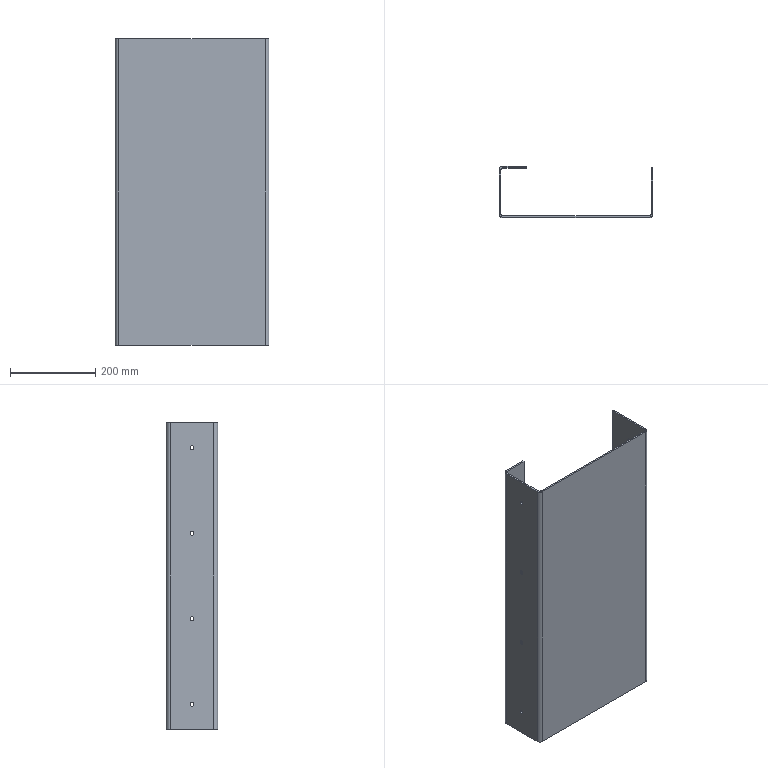Part | SolidWorks | features Extrusion 1, ICE 1 | 1 solid | 34 faces | box 360 x 120 x 716 mm | volume 1828022 mm3 | cylinder 22 | plane 12 | commonest cylinder face diameters 9 x16 10 x3 18 x3
STEP:
#1=CARTESIAN_POINT('',(296.,-55.5,58.));
#2=VERTEX_POINT('',#1);
#3=CARTESIAN_POINT('',(296.,-64.5,58.));
#4=VERTEX_POINT('',#3);
#5=CARTESIAN_POINT('',(296.,-60.,58.));
#6=DIRECTION('',(-1.,0.,0.));
#7=DIRECTION('',(0.,0.,1.));
#8=AXIS2_PLACEMENT_3D('',#5,#6,#7);
#9=CIRCLE('',#8,4.5);
#10=EDGE_CURVE('',#2,#4,#9,.T.);
#11=ORIENTED_EDGE('',*,*,#10,.F.);
#12=CARTESIAN_POINT('',(292.,-55.5,58.));
#13=VERTEX_POINT('',#12);
#14=CARTESIAN_POINT('',(652.,-55.5,58.));
#15=DIRECTION('',(-1.,0.,0.));
#16=VECTOR('',#15,1000.);
#17=LINE('',#14,#16);
#18=EDGE_CURVE('',#2,#13,#17,.T.);
#19=ORIENTED_EDGE('',*,*,#18,.T.);
#20=CARTESIAN_POINT('',(292.,-64.5,58.));
#21=VERTEX_POINT('',#20);
#22=CARTESIAN_POINT('',(292.,-60.,58.));
#23=DIRECTION('',(-1.,0.,0.));
#24=DIRECTION('',(0.,0.,1.));
#25=AXIS2_PLACEMENT_3D('',#22,#23,#24);
#26=CIRCLE('',#25,4.5);
#27=EDGE_CURVE('',#13,#21,#26,.T.);
#28=ORIENTED_EDGE('',*,*,#27,.T.);
#29=CARTESIAN_POINT('',(652.,-64.5,58.));
#30=DIRECTION('',(-1.,0.,0.));
#31=VECTOR('',#30,1000.);
#32=LINE('',#29,#31);
#33=EDGE_CURVE('',#4,#21,#32,.T.);
#34=ORIENTED_EDGE('',*,*,#33,.F.);
#35=EDGE_LOOP('',(#11,#19,#28,#34));
#36=FACE_OUTER_BOUND('',#35,.T.);
#37=CARTESIAN_POINT('',(652.,-60.,58.));
#38=DIRECTION('',(-1.,0.,0.));
#39=DIRECTION('',(0.,-1.,0.));
#40=AXIS2_PLACEMENT_3D('',#37,#38,#39);
#41=CYLINDRICAL_SURFACE('',#40,4.5);
#42=ADVANCED_FACE('',(#36),#41,.F.);
#43=CARTESIAN_POINT('',(296.,-55.5,258.));
#44=VERTEX_POINT('',#43);
#45=CARTESIAN_POINT('',(296.,-64.5,258.));
#46=VERTEX_POINT('',#45);
#47=CARTESIAN_POINT('',(296.,-60.,258.));
#48=DIRECTION('',(-1.,0.,0.));
#49=DIRECTION('',(0.,0.,1.));
#50=AXIS2_PLACEMENT_3D('',#47,#48,#49);
#51=CIRCLE('',#50,4.5);
#52=EDGE_CURVE('',#44,#46,#51,.T.);
#53=ORIENTED_EDGE('',*,*,#52,.F.);
#54=CARTESIAN_POINT('',(292.,-55.5,258.));
#55=VERTEX_POINT('',#54);
#56=CARTESIAN_POINT('',(652.,-55.5,258.));
#57=DIRECTION('',(-1.,0.,0.));
#58=VECTOR('',#57,1000.);
#59=LINE('',#56,#58);
#60=EDGE_CURVE('',#44,#55,#59,.T.);
#61=ORIENTED_EDGE('',*,*,#60,.T.);
#62=CARTESIAN_POINT('',(292.,-64.5,258.));
#63=VERTEX_POINT('',#62);
#64=CARTESIAN_POINT('',(292.,-60.,258.));
#65=DIRECTION('',(-1.,0.,0.));
#66=DIRECTION('',(0.,0.,1.));
#67=AXIS2_PLACEMENT_3D('',#64,#65,#66);
#68=CIRCLE('',#67,4.5);
#69=EDGE_CURVE('',#55,#63,#68,.T.);
#70=ORIENTED_EDGE('',*,*,#69,.T.);
#71=CARTESIAN_POINT('',(652.,-64.5,258.));
#72=DIRECTION('',(-1.,0.,0.));
#73=VECTOR('',#72,1000.);
#74=LINE('',#71,#73);
#75=EDGE_CURVE('',#46,#63,#74,.T.);
#76=ORIENTED_EDGE('',*,*,#75,.F.);
#77=EDGE_LOOP('',(#53,#61,#70,#76));
#78=FACE_OUTER_BOUND('',#77,.T.);
#79=CARTESIAN_POINT('',(652.,-60.,258.));
#80=DIRECTION('',(-1.,0.,0.));
#81=DIRECTION('',(0.,-1.,0.));
#82=AXIS2_PLACEMENT_3D('',#79,#80,#81);
#83=CYLINDRICAL_SURFACE('',#82,4.5);
#84=ADVANCED_FACE('',(#78),#83,.F.);
#85=CARTESIAN_POINT('',(296.,-55.5,458.));
#86=VERTEX_POINT('',#85);
#87=CARTESIAN_POINT('',(296.,-64.5,458.));
#88=VERTEX_POINT('',#87);
#89=CARTESIAN_POINT('',(296.,-60.,458.));
#90=DIRECTION('',(-1.,0.,0.));
#91=DIRECTION('',(0.,0.,1.));
#92=AXIS2_PLACEMENT_3D('',#89,#90,#91);
#93=CIRCLE('',#92,4.5);
#94=EDGE_CURVE('',#86,#88,#93,.T.);
#95=ORIENTED_EDGE('',*,*,#94,.F.);
#96=CARTESIAN_POINT('',(292.,-55.5,458.));
#97=VERTEX_POINT('',#96);
#98=CARTESIAN_POINT('',(652.,-55.5,458.));
#99=DIRECTION('',(-1.,0.,0.));
#100=VECTOR('',#99,1000.);
#101=LINE('',#98,#100);
#102=EDGE_CURVE('',#86,#97,#101,.T.);
#103=ORIENTED_EDGE('',*,*,#102,.T.);
#104=CARTESIAN_POINT('',(292.,-64.5,458.));
#105=VERTEX_POINT('',#104);
#106=CARTESIAN_POINT('',(292.,-60.,458.));
#107=DIRECTION('',(-1.,0.,0.));
#108=DIRECTION('',(0.,0.,1.));
#109=AXIS2_PLACEMENT_3D('',#106,#107,#108);
#110=CIRCLE('',#109,4.5);
#111=EDGE_CURVE('',#97,#105,#110,.T.);
#112=ORIENTED_EDGE('',*,*,#111,.T.);
#113=CARTESIAN_POINT('',(652.,-64.5,458.));
#114=DIRECTION('',(-1.,0.,0.));
#115=VECTOR('',#114,1000.);
#116=LINE('',#113,#115);
#117=EDGE_CURVE('',#88,#105,#116,.T.);
#118=ORIENTED_EDGE('',*,*,#117,.F.);
#119=EDGE_LOOP('',(#95,#103,#112,#118));
#120=FACE_OUTER_BOUND('',#119,.T.);
#121=CARTESIAN_POINT('',(652.,-60.,458.));
#122=DIRECTION('',(-1.,0.,0.));
#123=DIRECTION('',(0.,-1.,0.));
#124=AXIS2_PLACEMENT_3D('',#121,#122,#123);
#125=CYLINDRICAL_SURFACE('',#124,4.5);
#126=ADVANCED_FACE('',(#120),#125,.F.);
#127=CARTESIAN_POINT('',(296.,-55.5,658.));
#128=VERTEX_POINT('',#127);
#129=CARTESIAN_POINT('',(296.,-64.5,658.));
#130=VERTEX_POINT('',#129);
#131=CARTESIAN_POINT('',(296.,-60.,658.));
#132=DIRECTION('',(-1.,0.,0.));
#133=DIRECTION('',(0.,0.,1.));
#134=AXIS2_PLACEMENT_3D('',#131,#132,#133);
#135=CIRCLE('',#134,4.5);
#136=EDGE_CURVE('',#128,#130,#135,.T.);
#137=ORIENTED_EDGE('',*,*,#136,.F.);
#138=CARTESIAN_POINT('',(292.,-55.5,658.));
#139=VERTEX_POINT('',#138);
#140=CARTESIAN_POINT('',(652.,-55.5,658.));
#141=DIRECTION('',(-1.,0.,0.));
#142=VECTOR('',#141,1000.);
#143=LINE('',#140,#142);
#144=EDGE_CURVE('',#128,#139,#143,.T.);
#145=ORIENTED_EDGE('',*,*,#144,.T.);
#146=CARTESIAN_POINT('',(292.,-64.5,658.));
#147=VERTEX_POINT('',#146);
#148=CARTESIAN_POINT('',(292.,-60.,658.));
#149=DIRECTION('',(-1.,0.,0.));
#150=DIRECTION('',(0.,0.,1.));
#151=AXIS2_PLACEMENT_3D('',#148,#149,#150);
#152=CIRCLE('',#151,4.5);
#153=EDGE_CURVE('',#139,#147,#152,.T.);
#154=ORIENTED_EDGE('',*,*,#153,.T.);
#155=CARTESIAN_POINT('',(652.,-64.5,658.));
#156=DIRECTION('',(-1.,0.,0.));
#157=VECTOR('',#156,1000.);
#158=LINE('',#155,#157);
#159=EDGE_CURVE('',#130,#147,#158,.T.);
#160=ORIENTED_EDGE('',*,*,#159,.F.);
#161=EDGE_LOOP('',(#137,#145,#154,#160));
#162=FACE_OUTER_BOUND('',#161,.T.);
#163=CARTESIAN_POINT('',(652.,-60.,658.));
#164=DIRECTION('',(-1.,0.,0.));
#165=DIRECTION('',(0.,-1.,0.));
#166=AXIS2_PLACEMENT_3D('',#163,#164,#165);
#167=CYLINDRICAL_SURFACE('',#166,4.5);
#168=ADVANCED_FACE('',(#162),#167,.F.);
#169=CARTESIAN_POINT('',(-60.,-64.5,58.));
#170=VERTEX_POINT('',#169);
#171=CARTESIAN_POINT('',(-60.,-55.5,58.));
#172=VERTEX_POINT('',#171);
#173=CARTESIAN_POINT('',(-60.,-60.,58.));
#174=DIRECTION('',(1.,0.,0.));
#175=DIRECTION('',(0.,1.,0.));
#176=AXIS2_PLACEMENT_3D('',#173,#174,#175);
#177=CIRCLE('',#176,4.5);
#178=EDGE_CURVE('',#170,#172,#177,.T.);
#179=ORIENTED_EDGE('',*,*,#178,.T.);
#180=CARTESIAN_POINT('',(-64.,-55.5,58.));
#181=VERTEX_POINT('',#180);
#182=CARTESIAN_POINT('',(652.,-55.5,58.));
#183=DIRECTION('',(-1.,0.,0.));
#184=VECTOR('',#183,1000.);
#185=LINE('',#182,#184);
#186=EDGE_CURVE('',#172,#181,#185,.T.);
#187=ORIENTED_EDGE('',*,*,#186,.T.);
#188=CARTESIAN_POINT('',(-64.,-64.5,58.));
#189=VERTEX_POINT('',#188);
#190=CARTESIAN_POINT('',(-64.,-60.,58.));
#191=DIRECTION('',(-1.,0.,0.));
#192=DIRECTION('',(0.,-1.,0.));
#193=AXIS2_PLACEMENT_3D('',#190,#191,#192);
#194=CIRCLE('',#193,4.5);
#195=EDGE_CURVE('',#181,#189,#194,.T.);
#196=ORIENTED_EDGE('',*,*,#195,.T.);
#197=CARTESIAN_POINT('',(652.,-64.5,58.));
#198=DIRECTION('',(-1.,0.,0.));
#199=VECTOR('',#198,1000.);
#200=LINE('',#197,#199);
#201=EDGE_CURVE('',#170,#189,#200,.T.);
#202=ORIENTED_EDGE('',*,*,#201,.F.);
#203=EDGE_LOOP('',(#179,#187,#196,#202));
#204=FACE_OUTER_BOUND('',#203,.T.);
#205=CARTESIAN_POINT('',(652.,-60.,58.));
#206=DIRECTION('',(-1.,0.,0.));
#207=DIRECTION('',(0.,-1.,0.));
#208=AXIS2_PLACEMENT_3D('',#205,#206,#207);
#209=CYLINDRICAL_SURFACE('',#208,4.5);
#210=ADVANCED_FACE('',(#204),#209,.F.);
#211=CARTESIAN_POINT('',(-60.,-64.5,258.));
#212=VERTEX_POINT('',#211);
#213=CARTESIAN_POINT('',(-60.,-55.5,258.));
#214=VERTEX_POINT('',#213);
#215=CARTESIAN_POINT('',(-60.,-60.,258.));
#216=DIRECTION('',(1.,0.,0.));
#217=DIRECTION('',(0.,1.,0.));
#218=AXIS2_PLACEMENT_3D('',#215,#216,#217);
#219=CIRCLE('',#218,4.5);
#220=EDGE_CURVE('',#212,#214,#219,.T.);
#221=ORIENTED_EDGE('',*,*,#220,.T.);
#222=CARTESIAN_POINT('',(-64.,-55.5,258.));
#223=VERTEX_POINT('',#222);
#224=CARTESIAN_POINT('',(652.,-55.5,258.));
#225=DIRECTION('',(-1.,0.,0.));
#226=VECTOR('',#225,1000.);
#227=LINE('',#224,#226);
#228=EDGE_CURVE('',#214,#223,#227,.T.);
#229=ORIENTED_EDGE('',*,*,#228,.T.);
#230=CARTESIAN_POINT('',(-64.,-64.5,258.));
#231=VERTEX_POINT('',#230);
#232=CARTESIAN_POINT('',(-64.,-60.,258.));
#233=DIRECTION('',(-1.,0.,0.));
#234=DIRECTION('',(0.,-1.,0.));
#235=AXIS2_PLACEMENT_3D('',#232,#233,#234);
#236=CIRCLE('',#235,4.5);
#237=EDGE_CURVE('',#223,#231,#236,.T.);
#238=ORIENTED_EDGE('',*,*,#237,.T.);
#239=CARTESIAN_POINT('',(652.,-64.5,258.));
#240=DIRECTION('',(-1.,0.,0.));
#241=VECTOR('',#240,1000.);
#242=LINE('',#239,#241);
#243=EDGE_CURVE('',#212,#231,#242,.T.);
#244=ORIENTED_EDGE('',*,*,#243,.F.);
#245=EDGE_LOOP('',(#221,#229,#238,#244));
#246=FACE_OUTER_BOUND('',#245,.T.);
#247=CARTESIAN_POINT('',(652.,-60.,258.));
#248=DIRECTION('',(-1.,0.,0.));
#249=DIRECTION('',(0.,-1.,0.));
#250=AXIS2_PLACEMENT_3D('',#247,#248,#249);
#251=CYLINDRICAL_SURFACE('',#250,4.5);
#252=ADVANCED_FACE('',(#246),#251,.F.);
#253=CARTESIAN_POINT('',(-60.,-64.5,458.));
#254=VERTEX_POINT('',#253);
#255=CARTESIAN_POINT('',(-60.,-55.5,458.));
#256=VERTEX_POINT('',#255);
#257=CARTESIAN_POINT('',(-60.,-60.,458.));
#258=DIRECTION('',(1.,0.,0.));
#259=DIRECTION('',(0.,1.,0.));
#260=AXIS2_PLACEMENT_3D('',#257,#258,#259);
#261=CIRCLE('',#260,4.5);
#262=EDGE_CURVE('',#254,#256,#261,.T.);
#263=ORIENTED_EDGE('',*,*,#262,.T.);
#264=CARTESIAN_POINT('',(-64.,-55.5,458.));
#265=VERTEX_POINT('',#264);
#266=CARTESIAN_POINT('',(652.,-55.5,458.));
#267=DIRECTION('',(-1.,0.,0.));
#268=VECTOR('',#267,1000.);
#269=LINE('',#266,#268);
#270=EDGE_CURVE('',#256,#265,#269,.T.);
#271=ORIENTED_EDGE('',*,*,#270,.T.);
#272=CARTESIAN_POINT('',(-64.,-64.5,458.));
#273=VERTEX_POINT('',#272);
#274=CARTESIAN_POINT('',(-64.,-60.,458.));
#275=DIRECTION('',(-1.,0.,0.));
#276=DIRECTION('',(0.,-1.,0.));
#277=AXIS2_PLACEMENT_3D('',#274,#275,#276);
#278=CIRCLE('',#277,4.5);
#279=EDGE_CURVE('',#265,#273,#278,.T.);
#280=ORIENTED_EDGE('',*,*,#279,.T.);
#281=CARTESIAN_POINT('',(652.,-64.5,458.));
#282=DIRECTION('',(-1.,0.,0.));
#283=VECTOR('',#282,1000.);
#284=LINE('',#281,#283);
#285=EDGE_CURVE('',#254,#273,#284,.T.);
#286=ORIENTED_EDGE('',*,*,#285,.F.);
#287=EDGE_LOOP('',(#263,#271,#280,#286));
#288=FACE_OUTER_BOUND('',#287,.T.);
#289=CARTESIAN_POINT('',(652.,-60.,458.));
#290=DIRECTION('',(-1.,0.,0.));
#291=DIRECTION('',(0.,-1.,0.));
#292=AXIS2_PLACEMENT_3D('',#289,#290,#291);
#293=CYLINDRICAL_SURFACE('',#292,4.5);
#294=ADVANCED_FACE('',(#288),#293,.F.);
#295=CARTESIAN_POINT('',(-60.,-64.5,658.));
#296=VERTEX_POINT('',#295);
#297=CARTESIAN_POINT('',(-60.,-55.5,658.));
#298=VERTEX_POINT('',#297);
#299=CARTESIAN_POINT('',(-60.,-60.,658.));
#300=DIRECTION('',(1.,0.,0.));
#301=DIRECTION('',(0.,1.,0.));
#302=AXIS2_PLACEMENT_3D('',#299,#300,#301);
#303=CIRCLE('',#302,4.5);
#304=EDGE_CURVE('',#296,#298,#303,.T.);
#305=ORIENTED_EDGE('',*,*,#304,.T.);
#306=CARTESIAN_POINT('',(-64.,-55.5,658.));
#307=VERTEX_POINT('',#306);
#308=CARTESIAN_POINT('',(652.,-55.5,658.));
#309=DIRECTION('',(-1.,0.,0.));
#310=VECTOR('',#309,1000.);
#311=LINE('',#308,#310);
#312=EDGE_CURVE('',#298,#307,#311,.T.);
#313=ORIENTED_EDGE('',*,*,#312,.T.);
#314=CARTESIAN_POINT('',(-64.,-64.5,658.));
#315=VERTEX_POINT('',#314);
#316=CARTESIAN_POINT('',(-64.,-60.,658.));
#317=DIRECTION('',(-1.,0.,0.));
#318=DIRECTION('',(0.,-1.,0.));
#319=AXIS2_PLACEMENT_3D('',#316,#317,#318);
#320=CIRCLE('',#319,4.5);
#321=EDGE_CURVE('',#307,#315,#320,.T.);
#322=ORIENTED_EDGE('',*,*,#321,.T.);
#323=CARTESIAN_POINT('',(652.,-64.5,658.));
#324=DIRECTION('',(-1.,0.,0.));
#325=VECTOR('',#324,1000.);
#326=LINE('',#323,#325);
#327=EDGE_CURVE('',#296,#315,#326,.T.);
#328=ORIENTED_EDGE('',*,*,#327,.F.);
#329=EDGE_LOOP('',(#305,#313,#322,#328));
#330=FACE_OUTER_BOUND('',#329,.T.);
#331=CARTESIAN_POINT('',(652.,-60.,658.));
#332=DIRECTION('',(-1.,0.,0.));
#333=DIRECTION('',(0.,-1.,0.));
#334=AXIS2_PLACEMENT_3D('',#331,#332,#333);
#335=CYLINDRICAL_SURFACE('',#334,4.5);
#336=ADVANCED_FACE('',(#330),#335,.F.);
#337=CARTESIAN_POINT('',(296.,-60.,58.));
#338=DIRECTION('',(-1.,0.,0.));
#339=DIRECTION('',(0.,0.,1.));
#340=AXIS2_PLACEMENT_3D('',#337,#338,#339);
#341=CIRCLE('',#340,4.5);
#342=EDGE_CURVE('',#4,#2,#341,.T.);
#343=ORIENTED_EDGE('',*,*,#342,.T.);
#344=ORIENTED_EDGE('',*,*,#10,.T.);
#345=EDGE_LOOP('',(#343,#344));
#346=FACE_BOUND('',#345,.T.);
#347=CARTESIAN_POINT('',(296.,-60.,258.));
#348=DIRECTION('',(-1.,0.,0.));
#349=DIRECTION('',(0.,0.,1.));
#350=AXIS2_PLACEMENT_3D('',#347,#348,#349);
#351=CIRCLE('',#350,4.5);
#352=EDGE_CURVE('',#46,#44,#351,.T.);
#353=ORIENTED_EDGE('',*,*,#352,.T.);
#354=ORIENTED_EDGE('',*,*,#52,.T.);
#355=EDGE_LOOP('',(#353,#354));
#356=FACE_BOUND('',#355,.T.);
#357=CARTESIAN_POINT('',(296.,-60.,458.));
#358=DIRECTION('',(-1.,0.,0.));
#359=DIRECTION('',(0.,0.,1.));
#360=AXIS2_PLACEMENT_3D('',#357,#358,#359);
#361=CIRCLE('',#360,4.5);
#362=EDGE_CURVE('',#88,#86,#361,.T.);
#363=ORIENTED_EDGE('',*,*,#362,.T.);
#364=ORIENTED_EDGE('',*,*,#94,.T.);
#365=EDGE_LOOP('',(#363,#364));
#366=FACE_BOUND('',#365,.T.);
#367=CARTESIAN_POINT('',(296.,-60.,658.));
#368=DIRECTION('',(-1.,0.,0.));
#369=DIRECTION('',(0.,0.,1.));
#370=AXIS2_PLACEMENT_3D('',#367,#368,#369);
#371=CIRCLE('',#370,4.5);
#372=EDGE_CURVE('',#130,#128,#371,.T.);
#373=ORIENTED_EDGE('',*,*,#372,.T.);
#374=ORIENTED_EDGE('',*,*,#136,.T.);
#375=EDGE_LOOP('',(#373,#374));
#376=FACE_BOUND('',#375,.T.);
#377=CARTESIAN_POINT('',(296.,-111.,0.));
#378=VERTEX_POINT('',#377);
#379=CARTESIAN_POINT('',(296.,-4.,0.));
#380=VERTEX_POINT('',#379);
#381=CARTESIAN_POINT('',(296.,-111.,0.));
#382=DIRECTION('',(0.,1.,0.));
#383=VECTOR('',#382,1000.);
#384=LINE('',#381,#383);
#385=EDGE_CURVE('',#378,#380,#384,.T.);
#386=ORIENTED_EDGE('',*,*,#385,.T.);
#387=CARTESIAN_POINT('',(296.,-4.,716.));
#388=VERTEX_POINT('',#387);
#389=CARTESIAN_POINT('',(296.,-4.,716.));
#390=DIRECTION('',(0.,0.,-1.));
#391=VECTOR('',#390,1000.);
#392=LINE('',#389,#391);
#393=EDGE_CURVE('',#388,#380,#392,.T.);
#394=ORIENTED_EDGE('',*,*,#393,.F.);
#395=CARTESIAN_POINT('',(296.,-111.,716.));
#396=VERTEX_POINT('',#395);
#397=CARTESIAN_POINT('',(296.,-111.,716.));
#398=DIRECTION('',(0.,1.,0.));
#399=VECTOR('',#398,1000.);
#400=LINE('',#397,#399);
#401=EDGE_CURVE('',#396,#388,#400,.T.);
#402=ORIENTED_EDGE('',*,*,#401,.F.);
#403=CARTESIAN_POINT('',(296.,-111.,716.));
#404=DIRECTION('',(0.,0.,-1.));
#405=VECTOR('',#404,1000.);
#406=LINE('',#403,#405);
#407=EDGE_CURVE('',#396,#378,#406,.T.);
#408=ORIENTED_EDGE('',*,*,#407,.T.);
#409=EDGE_LOOP('',(#386,#394,#402,#408));
#410=FACE_OUTER_BOUND('',#409,.T.);
#411=CARTESIAN_POINT('',(296.,-111.,716.));
#412=DIRECTION('',(-1.,0.,0.));
#413=DIRECTION('',(0.,0.,1.));
#414=AXIS2_PLACEMENT_3D('',#411,#412,#413);
#415=PLANE('',#414);
#416=ADVANCED_FACE('',(#346,#356,#366,#376,#410),#415,.F.);
#417=CARTESIAN_POINT('',(292.,-4.,0.));
#418=VERTEX_POINT('',#417);
#419=CARTESIAN_POINT('',(296.,-4.,0.));
#420=DIRECTION('',(-1.,0.,0.));
#421=VECTOR('',#420,1000.);
#422=LINE('',#419,#421);
#423=EDGE_CURVE('',#380,#418,#422,.T.);
#424=ORIENTED_EDGE('',*,*,#423,.T.);
#425=CARTESIAN_POINT('',(292.,-4.,716.));
#426=VERTEX_POINT('',#425);
#427=CARTESIAN_POINT('',(292.,-4.,716.));
#428=DIRECTION('',(0.,0.,-1.));
#429=VECTOR('',#428,1000.);
#430=LINE('',#427,#429);
#431=EDGE_CURVE('',#426,#418,#430,.T.);
#432=ORIENTED_EDGE('',*,*,#431,.F.);
#433=CARTESIAN_POINT('',(296.,-4.,716.));
#434=DIRECTION('',(-1.,0.,0.));
#435=VECTOR('',#434,1000.);
#436=LINE('',#433,#435);
#437=EDGE_CURVE('',#388,#426,#436,.T.);
#438=ORIENTED_EDGE('',*,*,#437,.F.);
#439=ORIENTED_EDGE('',*,*,#393,.T.);
#440=EDGE_LOOP('',(#424,#432,#438,#439));
#441=FACE_OUTER_BOUND('',#440,.T.);
#442=CARTESIAN_POINT('',(296.,-4.,716.));
#443=DIRECTION('',(0.,-1.,0.));
#444=DIRECTION('',(0.,0.,-1.));
#445=AXIS2_PLACEMENT_3D('',#442,#443,#444);
#446=PLANE('',#445);
#447=ADVANCED_FACE('',(#441),#446,.F.);
#448=CARTESIAN_POINT('',(292.,-60.,58.));
#449=DIRECTION('',(-1.,0.,0.));
#450=DIRECTION('',(0.,0.,1.));
#451=AXIS2_PLACEMENT_3D('',#448,#449,#450);
#452=CIRCLE('',#451,4.5);
#453=EDGE_CURVE('',#21,#13,#452,.T.);
#454=ORIENTED_EDGE('',*,*,#453,.F.);
#455=ORIENTED_EDGE('',*,*,#27,.F.);
#456=EDGE_LOOP('',(#454,#455));
#457=FACE_BOUND('',#456,.T.);
#458=CARTESIAN_POINT('',(292.,-60.,258.));
#459=DIRECTION('',(-1.,0.,0.));
#460=DIRECTION('',(0.,0.,1.));
#461=AXIS2_PLACEMENT_3D('',#458,#459,#460);
#462=CIRCLE('',#461,4.5);
#463=EDGE_CURVE('',#63,#55,#462,.T.);
#464=ORIENTED_EDGE('',*,*,#463,.F.);
#465=ORIENTED_EDGE('',*,*,#69,.F.);
#466=EDGE_LOOP('',(#464,#465));
#467=FACE_BOUND('',#466,.T.);
#468=CARTESIAN_POINT('',(292.,-60.,458.));
#469=DIRECTION('',(-1.,0.,0.));
#470=DIRECTION('',(0.,0.,1.));
#471=AXIS2_PLACEMENT_3D('',#468,#469,#470);
#472=CIRCLE('',#471,4.5);
#473=EDGE_CURVE('',#105,#97,#472,.T.);
#474=ORIENTED_EDGE('',*,*,#473,.F.);
#475=ORIENTED_EDGE('',*,*,#111,.F.);
#476=EDGE_LOOP('',(#474,#475));
#477=FACE_BOUND('',#476,.T.);
#478=CARTESIAN_POINT('',(292.,-60.,658.));
#479=DIRECTION('',(-1.,0.,0.));
#480=DIRECTION('',(0.,0.,1.));
#481=AXIS2_PLACEMENT_3D('',#478,#479,#480);
#482=CIRCLE('',#481,4.5);
#483=EDGE_CURVE('',#147,#139,#482,.T.);
#484=ORIENTED_EDGE('',*,*,#483,.F.);
#485=ORIENTED_EDGE('',*,*,#153,.F.);
#486=EDGE_LOOP('',(#484,#485));
#487=FACE_BOUND('',#486,.T.);
#488=CARTESIAN_POINT('',(292.,-111.,0.));
#489=VERTEX_POINT('',#488);
#490=CARTESIAN_POINT('',(292.,-111.,0.));
#491=DIRECTION('',(0.,1.,0.));
#492=VECTOR('',#491,1000.);
#493=LINE('',#490,#492);
#494=EDGE_CURVE('',#489,#418,#493,.T.);
#495=ORIENTED_EDGE('',*,*,#494,.F.);
#496=CARTESIAN_POINT('',(292.,-111.,716.));
#497=VERTEX_POINT('',#496);
#498=CARTESIAN_POINT('',(292.,-111.,716.));
#499=DIRECTION('',(0.,0.,-1.));
#500=VECTOR('',#499,1000.);
#501=LINE('',#498,#500);
#502=EDGE_CURVE('',#497,#489,#501,.T.);
#503=ORIENTED_EDGE('',*,*,#502,.F.);
#504=CARTESIAN_POINT('',(292.,-111.,716.));
#505=DIRECTION('',(0.,1.,0.));
#506=VECTOR('',#505,1000.);
#507=LINE('',#504,#506);
#508=EDGE_CURVE('',#497,#426,#507,.T.);
#509=ORIENTED_EDGE('',*,*,#508,.T.);
#510=ORIENTED_EDGE('',*,*,#431,.T.);
#511=EDGE_LOOP('',(#495,#503,#509,#510));
#512=FACE_OUTER_BOUND('',#511,.T.);
#513=CARTESIAN_POINT('',(292.,-111.,716.));
#514=DIRECTION('',(-1.,0.,0.));
#515=DIRECTION('',(0.,0.,1.));
#516=AXIS2_PLACEMENT_3D('',#513,#514,#515);
#517=PLANE('',#516);
#518=ADVANCED_FACE('',(#457,#467,#477,#487,#512),#517,.T.);
#519=CARTESIAN_POINT('',(287.,-116.,0.));
#520=VERTEX_POINT('',#519);
#521=CARTESIAN_POINT('',(287.,-111.,0.));
#522=DIRECTION('',(0.,0.,1.));
#523=DIRECTION('',(1.,0.,0.));
#524=AXIS2_PLACEMENT_3D('',#521,#522,#523);
#525=CIRCLE('',#524,5.);
#526=EDGE_CURVE('',#520,#489,#525,.T.);
#527=ORIENTED_EDGE('',*,*,#526,.F.);
#528=CARTESIAN_POINT('',(287.,-116.,716.));
#529=VERTEX_POINT('',#528);
#530=CARTESIAN_POINT('',(287.,-116.,716.));
#531=DIRECTION('',(0.,0.,-1.));
#532=VECTOR('',#531,1000.);
#533=LINE('',#530,#532);
#534=EDGE_CURVE('',#529,#520,#533,.T.);
#535=ORIENTED_EDGE('',*,*,#534,.F.);
#536=CARTESIAN_POINT('',(287.,-111.,716.));
#537=DIRECTION('',(0.,0.,1.));
#538=DIRECTION('',(1.,0.,0.));
#539=AXIS2_PLACEMENT_3D('',#536,#537,#538);
#540=CIRCLE('',#539,5.);
#541=EDGE_CURVE('',#529,#497,#540,.T.);
#542=ORIENTED_EDGE('',*,*,#541,.T.);
#543=ORIENTED_EDGE('',*,*,#502,.T.);
#544=EDGE_LOOP('',(#527,#535,#542,#543));
#545=FACE_OUTER_BOUND('',#544,.T.);
#546=CARTESIAN_POINT('',(287.,-111.,716.));
#547=DIRECTION('',(0.,0.,-1.));
#548=DIRECTION('',(-1.,0.,0.));
#549=AXIS2_PLACEMENT_3D('',#546,#547,#548);
#550=CYLINDRICAL_SURFACE('',#549,5.);
#551=ADVANCED_FACE('',(#545),#550,.F.);
#552=CARTESIAN_POINT('',(-55.,-116.,0.));
#553=VERTEX_POINT('',#552);
#554=CARTESIAN_POINT('',(-55.,-116.,0.));
#555=DIRECTION('',(1.,0.,0.));
#556=VECTOR('',#555,1000.);
#557=LINE('',#554,#556);
#558=EDGE_CURVE('',#553,#520,#557,.T.);
#559=ORIENTED_EDGE('',*,*,#558,.F.);
#560=CARTESIAN_POINT('',(-55.,-116.,716.));
#561=VERTEX_POINT('',#560);
#562=CARTESIAN_POINT('',(-55.,-116.,716.));
#563=DIRECTION('',(0.,0.,-1.));
#564=VECTOR('',#563,1000.);
#565=LINE('',#562,#564);
#566=EDGE_CURVE('',#561,#553,#565,.T.);
#567=ORIENTED_EDGE('',*,*,#566,.F.);
#568=CARTESIAN_POINT('',(-55.,-116.,716.));
#569=DIRECTION('',(1.,0.,0.));
#570=VECTOR('',#569,1000.);
#571=LINE('',#568,#570);
#572=EDGE_CURVE('',#561,#529,#571,.T.);
#573=ORIENTED_EDGE('',*,*,#572,.T.);
#574=ORIENTED_EDGE('',*,*,#534,.T.);
#575=EDGE_LOOP('',(#559,#567,#573,#574));
#576=FACE_OUTER_BOUND('',#575,.T.);
#577=CARTESIAN_POINT('',(-55.,-116.,716.));
#578=DIRECTION('',(0.,1.,0.));
#579=DIRECTION('',(-1.,0.,0.));
#580=AXIS2_PLACEMENT_3D('',#577,#578,#579);
#581=PLANE('',#580);
#582=ADVANCED_FACE('',(#576),#581,.T.);
#583=CARTESIAN_POINT('',(-60.,-111.,0.));
#584=VERTEX_POINT('',#583);
#585=CARTESIAN_POINT('',(-55.,-111.,0.));
#586=DIRECTION('',(0.,0.,1.));
#587=DIRECTION('',(1.,0.,0.));
#588=AXIS2_PLACEMENT_3D('',#585,#586,#587);
#589=CIRCLE('',#588,5.);
#590=EDGE_CURVE('',#584,#553,#589,.T.);
#591=ORIENTED_EDGE('',*,*,#590,.F.);
#592=CARTESIAN_POINT('',(-60.,-111.,716.));
#593=VERTEX_POINT('',#592);
#594=CARTESIAN_POINT('',(-60.,-111.,716.));
#595=DIRECTION('',(0.,0.,-1.));
#596=VECTOR('',#595,1000.);
#597=LINE('',#594,#596);
#598=EDGE_CURVE('',#593,#584,#597,.T.);
#599=ORIENTED_EDGE('',*,*,#598,.F.);
#600=CARTESIAN_POINT('',(-55.,-111.,716.));
#601=DIRECTION('',(0.,0.,1.));
#602=DIRECTION('',(1.,0.,0.));
#603=AXIS2_PLACEMENT_3D('',#600,#601,#602);
#604=CIRCLE('',#603,5.);
#605=EDGE_CURVE('',#593,#561,#604,.T.);
#606=ORIENTED_EDGE('',*,*,#605,.T.);
#607=ORIENTED_EDGE('',*,*,#566,.T.);
#608=EDGE_LOOP('',(#591,#599,#606,#607));
#609=FACE_OUTER_BOUND('',#608,.T.);
#610=CARTESIAN_POINT('',(-55.,-111.,716.));
#611=DIRECTION('',(0.,0.,-1.));
#612=DIRECTION('',(-1.,0.,0.));
#613=AXIS2_PLACEMENT_3D('',#610,#611,#612);
#614=CYLINDRICAL_SURFACE('',#613,5.);
#615=ADVANCED_FACE('',(#609),#614,.F.);
#616=ORIENTED_EDGE('',*,*,#178,.F.);
#617=CARTESIAN_POINT('',(-60.,-60.,58.));
#618=DIRECTION('',(1.,0.,0.));
#619=DIRECTION('',(0.,1.,0.));
#620=AXIS2_PLACEMENT_3D('',#617,#618,#619);
#621=CIRCLE('',#620,4.5);
#622=EDGE_CURVE('',#172,#170,#621,.T.);
#623=ORIENTED_EDGE('',*,*,#622,.F.);
#624=EDGE_LOOP('',(#616,#623));
#625=FACE_BOUND('',#624,.T.);
#626=ORIENTED_EDGE('',*,*,#220,.F.);
#627=CARTESIAN_POINT('',(-60.,-60.,258.));
#628=DIRECTION('',(1.,0.,0.));
#629=DIRECTION('',(0.,1.,0.));
#630=AXIS2_PLACEMENT_3D('',#627,#628,#629);
#631=CIRCLE('',#630,4.5);
#632=EDGE_CURVE('',#214,#212,#631,.T.);
#633=ORIENTED_EDGE('',*,*,#632,.F.);
#634=EDGE_LOOP('',(#626,#633));
#635=FACE_BOUND('',#634,.T.);
#636=ORIENTED_EDGE('',*,*,#262,.F.);
#637=CARTESIAN_POINT('',(-60.,-60.,458.));
#638=DIRECTION('',(1.,0.,0.));
#639=DIRECTION('',(0.,1.,0.));
#640=AXIS2_PLACEMENT_3D('',#637,#638,#639);
#641=CIRCLE('',#640,4.5);
#642=EDGE_CURVE('',#256,#254,#641,.T.);
#643=ORIENTED_EDGE('',*,*,#642,.F.);
#644=EDGE_LOOP('',(#636,#643));
#645=FACE_BOUND('',#644,.T.);
#646=ORIENTED_EDGE('',*,*,#304,.F.);
#647=CARTESIAN_POINT('',(-60.,-60.,658.));
#648=DIRECTION('',(1.,0.,0.));
#649=DIRECTION('',(0.,1.,0.));
#650=AXIS2_PLACEMENT_3D('',#647,#648,#649);
#651=CIRCLE('',#650,4.5);
#652=EDGE_CURVE('',#298,#296,#651,.T.);
#653=ORIENTED_EDGE('',*,*,#652,.F.);
#654=EDGE_LOOP('',(#646,#653));
#655=FACE_BOUND('',#654,.T.);
#656=CARTESIAN_POINT('',(-60.,-9.,0.));
#657=VERTEX_POINT('',#656);
#658=CARTESIAN_POINT('',(-60.,-9.,0.));
#659=DIRECTION('',(0.,-1.,0.));
#660=VECTOR('',#659,1000.);
#661=LINE('',#658,#660);
#662=EDGE_CURVE('',#657,#584,#661,.T.);
#663=ORIENTED_EDGE('',*,*,#662,.F.);
#664=CARTESIAN_POINT('',(-60.,-9.,716.));
#665=VERTEX_POINT('',#664);
#666=CARTESIAN_POINT('',(-60.,-9.,716.));
#667=DIRECTION('',(0.,0.,-1.));
#668=VECTOR('',#667,1000.);
#669=LINE('',#666,#668);
#670=EDGE_CURVE('',#665,#657,#669,.T.);
#671=ORIENTED_EDGE('',*,*,#670,.F.);
#672=CARTESIAN_POINT('',(-60.,-9.,716.));
#673=DIRECTION('',(0.,-1.,0.));
#674=VECTOR('',#673,1000.);
#675=LINE('',#672,#674);
#676=EDGE_CURVE('',#665,#593,#675,.T.);
#677=ORIENTED_EDGE('',*,*,#676,.T.);
#678=ORIENTED_EDGE('',*,*,#598,.T.);
#679=EDGE_LOOP('',(#663,#671,#677,#678));
#680=FACE_OUTER_BOUND('',#679,.T.);
#681=CARTESIAN_POINT('',(-60.,-9.,716.));
#682=DIRECTION('',(1.,0.,0.));
#683=DIRECTION('',(0.,1.,0.));
#684=AXIS2_PLACEMENT_3D('',#681,#682,#683);
#685=PLANE('',#684);
#686=ADVANCED_FACE('',(#625,#635,#645,#655,#680),#685,.T.);
#687=CARTESIAN_POINT('',(-55.,-4.,0.));
#688=VERTEX_POINT('',#687);
#689=CARTESIAN_POINT('',(-55.,-9.,0.));
#690=DIRECTION('',(0.,0.,1.));
#691=DIRECTION('',(1.,0.,0.));
#692=AXIS2_PLACEMENT_3D('',#689,#690,#691);
#693=CIRCLE('',#692,5.);
#694=EDGE_CURVE('',#688,#657,#693,.T.);
#695=ORIENTED_EDGE('',*,*,#694,.F.);
#696=CARTESIAN_POINT('',(-55.,-4.,716.));
#697=VERTEX_POINT('',#696);
#698=CARTESIAN_POINT('',(-55.,-4.,716.));
#699=DIRECTION('',(0.,0.,-1.));
#700=VECTOR('',#699,1000.);
#701=LINE('',#698,#700);
#702=EDGE_CURVE('',#697,#688,#701,.T.);
#703=ORIENTED_EDGE('',*,*,#702,.F.);
#704=CARTESIAN_POINT('',(-55.,-9.,716.));
#705=DIRECTION('',(0.,0.,1.));
#706=DIRECTION('',(1.,0.,0.));
#707=AXIS2_PLACEMENT_3D('',#704,#705,#706);
#708=CIRCLE('',#707,5.);
#709=EDGE_CURVE('',#697,#665,#708,.T.);
#710=ORIENTED_EDGE('',*,*,#709,.T.);
#711=ORIENTED_EDGE('',*,*,#670,.T.);
#712=EDGE_LOOP('',(#695,#703,#710,#711));
#713=FACE_OUTER_BOUND('',#712,.T.);
#714=CARTESIAN_POINT('',(-55.,-9.,716.));
#715=DIRECTION('',(0.,0.,-1.));
#716=DIRECTION('',(-1.,0.,0.));
#717=AXIS2_PLACEMENT_3D('',#714,#715,#716);
#718=CYLINDRICAL_SURFACE('',#717,5.);
#719=ADVANCED_FACE('',(#713),#718,.F.);
#720=CARTESIAN_POINT('',(0.,-4.,0.));
#721=VERTEX_POINT('',#720);
#722=CARTESIAN_POINT('',(0.,-4.,0.));
#723=DIRECTION('',(-1.,0.,0.));
#724=VECTOR('',#723,1000.);
#725=LINE('',#722,#724);
#726=EDGE_CURVE('',#721,#688,#725,.T.);
#727=ORIENTED_EDGE('',*,*,#726,.F.);
#728=CARTESIAN_POINT('',(0.,-4.,716.));
#729=VERTEX_POINT('',#728);
#730=CARTESIAN_POINT('',(0.,-4.,716.));
#731=DIRECTION('',(0.,0.,-1.));
#732=VECTOR('',#731,1000.);
#733=LINE('',#730,#732);
#734=EDGE_CURVE('',#729,#721,#733,.T.);
#735=ORIENTED_EDGE('',*,*,#734,.F.);
#736=CARTESIAN_POINT('',(0.,-4.,716.));
#737=DIRECTION('',(-1.,0.,0.));
#738=VECTOR('',#737,1000.);
#739=LINE('',#736,#738);
#740=EDGE_CURVE('',#729,#697,#739,.T.);
#741=ORIENTED_EDGE('',*,*,#740,.T.);
#742=ORIENTED_EDGE('',*,*,#702,.T.);
#743=EDGE_LOOP('',(#727,#735,#741,#742));
#744=FACE_OUTER_BOUND('',#743,.T.);
#745=CARTESIAN_POINT('',(0.,-4.,716.));
#746=DIRECTION('',(0.,-1.,0.));
#747=DIRECTION('',(0.,0.,-1.));
#748=AXIS2_PLACEMENT_3D('',#745,#746,#747);
#749=PLANE('',#748);
#750=ADVANCED_FACE('',(#744),#749,.T.);
#751=CARTESIAN_POINT('',(0.,0.,0.));
#752=VERTEX_POINT('',#751);
#753=CARTESIAN_POINT('',(0.,0.,0.));
#754=DIRECTION('',(0.,-1.,0.));
#755=VECTOR('',#754,1000.);
#756=LINE('',#753,#755);
#757=EDGE_CURVE('',#752,#721,#756,.T.);
#758=ORIENTED_EDGE('',*,*,#757,.F.);
#759=CARTESIAN_POINT('',(0.,0.,716.));
#760=VERTEX_POINT('',#759);
#761=CARTESIAN_POINT('',(0.,0.,716.));
#762=DIRECTION('',(0.,0.,-1.));
#763=VECTOR('',#762,1000.);
#764=LINE('',#761,#763);
#765=EDGE_CURVE('',#760,#752,#764,.T.);
#766=ORIENTED_EDGE('',*,*,#765,.F.);
#767=CARTESIAN_POINT('',(0.,0.,716.));
#768=DIRECTION('',(0.,-1.,0.));
#769=VECTOR('',#768,1000.);
#770=LINE('',#767,#769);
#771=EDGE_CURVE('',#760,#729,#770,.T.);
#772=ORIENTED_EDGE('',*,*,#771,.T.);
#773=ORIENTED_EDGE('',*,*,#734,.T.);
#774=EDGE_LOOP('',(#758,#766,#772,#773));
#775=FACE_OUTER_BOUND('',#774,.T.);
#776=CARTESIAN_POINT('',(0.,0.,716.));
#777=DIRECTION('',(1.,0.,0.));
#778=DIRECTION('',(0.,0.,-1.));
#779=AXIS2_PLACEMENT_3D('',#776,#777,#778);
#780=PLANE('',#779);
#781=ADVANCED_FACE('',(#775),#780,.T.);
#782=CARTESIAN_POINT('',(-55.,0.,0.));
#783=VERTEX_POINT('',#782);
#784=CARTESIAN_POINT('',(0.,0.,0.));
#785=DIRECTION('',(-1.,0.,0.));
#786=VECTOR('',#785,1000.);
#787=LINE('',#784,#786);
#788=EDGE_CURVE('',#752,#783,#787,.T.);
#789=ORIENTED_EDGE('',*,*,#788,.T.);
#790=CARTESIAN_POINT('',(-55.,0.,716.));
#791=VERTEX_POINT('',#790);
#792=CARTESIAN_POINT('',(-55.,0.,716.));
#793=DIRECTION('',(0.,0.,-1.));
#794=VECTOR('',#793,1000.);
#795=LINE('',#792,#794);
#796=EDGE_CURVE('',#791,#783,#795,.T.);
#797=ORIENTED_EDGE('',*,*,#796,.F.);
#798=CARTESIAN_POINT('',(0.,0.,716.));
#799=DIRECTION('',(-1.,0.,0.));
#800=VECTOR('',#799,1000.);
#801=LINE('',#798,#800);
#802=EDGE_CURVE('',#760,#791,#801,.T.);
#803=ORIENTED_EDGE('',*,*,#802,.F.);
#804=ORIENTED_EDGE('',*,*,#765,.T.);
#805=EDGE_LOOP('',(#789,#797,#803,#804));
#806=FACE_OUTER_BOUND('',#805,.T.);
#807=CARTESIAN_POINT('',(0.,0.,716.));
#808=DIRECTION('',(0.,-1.,0.));
#809=DIRECTION('',(0.,0.,-1.));
#810=AXIS2_PLACEMENT_3D('',#807,#808,#809);
#811=PLANE('',#810);
#812=ADVANCED_FACE('',(#806),#811,.F.);
#813=CARTESIAN_POINT('',(-64.,-9.,0.));
#814=VERTEX_POINT('',#813);
#815=CARTESIAN_POINT('',(-55.,-9.,0.));
#816=DIRECTION('',(0.,0.,1.));
#817=DIRECTION('',(1.,0.,0.));
#818=AXIS2_PLACEMENT_3D('',#815,#816,#817);
#819=CIRCLE('',#818,9.);
#820=EDGE_CURVE('',#783,#814,#819,.T.);
#821=ORIENTED_EDGE('',*,*,#820,.T.);
#822=CARTESIAN_POINT('',(-64.,-9.,716.));
#823=VERTEX_POINT('',#822);
#824=CARTESIAN_POINT('',(-64.,-9.,716.));
#825=DIRECTION('',(0.,0.,-1.));
#826=VECTOR('',#825,1000.);
#827=LINE('',#824,#826);
#828=EDGE_CURVE('',#823,#814,#827,.T.);
#829=ORIENTED_EDGE('',*,*,#828,.F.);
#830=CARTESIAN_POINT('',(-55.,-9.,716.));
#831=DIRECTION('',(0.,0.,1.));
#832=DIRECTION('',(1.,0.,0.));
#833=AXIS2_PLACEMENT_3D('',#830,#831,#832);
#834=CIRCLE('',#833,9.);
#835=EDGE_CURVE('',#791,#823,#834,.T.);
#836=ORIENTED_EDGE('',*,*,#835,.F.);
#837=ORIENTED_EDGE('',*,*,#796,.T.);
#838=EDGE_LOOP('',(#821,#829,#836,#837));
#839=FACE_OUTER_BOUND('',#838,.T.);
#840=CARTESIAN_POINT('',(-55.,-9.,716.));
#841=DIRECTION('',(0.,0.,-1.));
#842=DIRECTION('',(-1.,0.,0.));
#843=AXIS2_PLACEMENT_3D('',#840,#841,#842);
#844=CYLINDRICAL_SURFACE('',#843,9.);
#845=ADVANCED_FACE('',(#839),#844,.T.);
#846=CARTESIAN_POINT('',(-64.,-60.,58.));
#847=DIRECTION('',(-1.,0.,0.));
#848=DIRECTION('',(0.,-1.,0.));
#849=AXIS2_PLACEMENT_3D('',#846,#847,#848);
#850=CIRCLE('',#849,4.5);
#851=EDGE_CURVE('',#189,#181,#850,.T.);
#852=ORIENTED_EDGE('',*,*,#851,.F.);
#853=ORIENTED_EDGE('',*,*,#195,.F.);
#854=EDGE_LOOP('',(#852,#853));
#855=FACE_BOUND('',#854,.T.);
#856=CARTESIAN_POINT('',(-64.,-60.,258.));
#857=DIRECTION('',(-1.,0.,0.));
#858=DIRECTION('',(0.,-1.,0.));
#859=AXIS2_PLACEMENT_3D('',#856,#857,#858);
#860=CIRCLE('',#859,4.5);
#861=EDGE_CURVE('',#231,#223,#860,.T.);
#862=ORIENTED_EDGE('',*,*,#861,.F.);
#863=ORIENTED_EDGE('',*,*,#237,.F.);
#864=EDGE_LOOP('',(#862,#863));
#865=FACE_BOUND('',#864,.T.);
#866=CARTESIAN_POINT('',(-64.,-60.,458.));
#867=DIRECTION('',(-1.,0.,0.));
#868=DIRECTION('',(0.,-1.,0.));
#869=AXIS2_PLACEMENT_3D('',#866,#867,#868);
#870=CIRCLE('',#869,4.5);
#871=EDGE_CURVE('',#273,#265,#870,.T.);
#872=ORIENTED_EDGE('',*,*,#871,.F.);
#873=ORIENTED_EDGE('',*,*,#279,.F.);
#874=EDGE_LOOP('',(#872,#873));
#875=FACE_BOUND('',#874,.T.);
#876=CARTESIAN_POINT('',(-64.,-60.,658.));
#877=DIRECTION('',(-1.,0.,0.));
#878=DIRECTION('',(0.,-1.,0.));
#879=AXIS2_PLACEMENT_3D('',#876,#877,#878);
#880=CIRCLE('',#879,4.5);
#881=EDGE_CURVE('',#315,#307,#880,.T.);
#882=ORIENTED_EDGE('',*,*,#881,.F.);
#883=ORIENTED_EDGE('',*,*,#321,.F.);
#884=EDGE_LOOP('',(#882,#883));
#885=FACE_BOUND('',#884,.T.);
#886=CARTESIAN_POINT('',(-64.,-111.,0.));
#887=VERTEX_POINT('',#886);
#888=CARTESIAN_POINT('',(-64.,-9.,0.));
#889=DIRECTION('',(0.,-1.,0.));
#890=VECTOR('',#889,1000.);
#891=LINE('',#888,#890);
#892=EDGE_CURVE('',#814,#887,#891,.T.);
#893=ORIENTED_EDGE('',*,*,#892,.T.);
#894=CARTESIAN_POINT('',(-64.,-111.,716.));
#895=VERTEX_POINT('',#894);
#896=CARTESIAN_POINT('',(-64.,-111.,716.));
#897=DIRECTION('',(0.,0.,-1.));
#898=VECTOR('',#897,1000.);
#899=LINE('',#896,#898);
#900=EDGE_CURVE('',#895,#887,#899,.T.);
#901=ORIENTED_EDGE('',*,*,#900,.F.);
#902=CARTESIAN_POINT('',(-64.,-9.,716.));
#903=DIRECTION('',(0.,-1.,0.));
#904=VECTOR('',#903,1000.);
#905=LINE('',#902,#904);
#906=EDGE_CURVE('',#823,#895,#905,.T.);
#907=ORIENTED_EDGE('',*,*,#906,.F.);
#908=ORIENTED_EDGE('',*,*,#828,.T.);
#909=EDGE_LOOP('',(#893,#901,#907,#908));
#910=FACE_OUTER_BOUND('',#909,.T.);
#911=CARTESIAN_POINT('',(-64.,-9.,716.));
#912=DIRECTION('',(1.,0.,0.));
#913=DIRECTION('',(0.,0.,-1.));
#914=AXIS2_PLACEMENT_3D('',#911,#912,#913);
#915=PLANE('',#914);
#916=ADVANCED_FACE('',(#855,#865,#875,#885,#910),#915,.F.);
#917=CARTESIAN_POINT('',(-55.,-120.,0.));
#918=VERTEX_POINT('',#917);
#919=CARTESIAN_POINT('',(-55.,-111.,0.));
#920=DIRECTION('',(0.,0.,1.));
#921=DIRECTION('',(1.,0.,0.));
#922=AXIS2_PLACEMENT_3D('',#919,#920,#921);
#923=CIRCLE('',#922,9.);
#924=EDGE_CURVE('',#887,#918,#923,.T.);
#925=ORIENTED_EDGE('',*,*,#924,.T.);
#926=CARTESIAN_POINT('',(-55.,-120.,716.));
#927=VERTEX_POINT('',#926);
#928=CARTESIAN_POINT('',(-55.,-120.,716.));
#929=DIRECTION('',(0.,0.,-1.));
#930=VECTOR('',#929,1000.);
#931=LINE('',#928,#930);
#932=EDGE_CURVE('',#927,#918,#931,.T.);
#933=ORIENTED_EDGE('',*,*,#932,.F.);
#934=CARTESIAN_POINT('',(-55.,-111.,716.));
#935=DIRECTION('',(0.,0.,1.));
#936=DIRECTION('',(1.,0.,0.));
#937=AXIS2_PLACEMENT_3D('',#934,#935,#936);
#938=CIRCLE('',#937,9.);
#939=EDGE_CURVE('',#895,#927,#938,.T.);
#940=ORIENTED_EDGE('',*,*,#939,.F.);
#941=ORIENTED_EDGE('',*,*,#900,.T.);
#942=EDGE_LOOP('',(#925,#933,#940,#941));
#943=FACE_OUTER_BOUND('',#942,.T.);
#944=CARTESIAN_POINT('',(-55.,-111.,716.));
#945=DIRECTION('',(0.,0.,-1.));
#946=DIRECTION('',(-1.,0.,0.));
#947=AXIS2_PLACEMENT_3D('',#944,#945,#946);
#948=CYLINDRICAL_SURFACE('',#947,9.);
#949=ADVANCED_FACE('',(#943),#948,.T.);
#950=CARTESIAN_POINT('',(287.,-120.,0.));
#951=VERTEX_POINT('',#950);
#952=CARTESIAN_POINT('',(-55.,-120.,0.));
#953=DIRECTION('',(1.,0.,0.));
#954=VECTOR('',#953,1000.);
#955=LINE('',#952,#954);
#956=EDGE_CURVE('',#918,#951,#955,.T.);
#957=ORIENTED_EDGE('',*,*,#956,.T.);
#958=CARTESIAN_POINT('',(287.,-120.,716.));
#959=VERTEX_POINT('',#958);
#960=CARTESIAN_POINT('',(287.,-120.,716.));
#961=DIRECTION('',(0.,0.,-1.));
#962=VECTOR('',#961,1000.);
#963=LINE('',#960,#962);
#964=EDGE_CURVE('',#959,#951,#963,.T.);
#965=ORIENTED_EDGE('',*,*,#964,.F.);
#966=CARTESIAN_POINT('',(-55.,-120.,716.));
#967=DIRECTION('',(1.,0.,0.));
#968=VECTOR('',#967,1000.);
#969=LINE('',#966,#968);
#970=EDGE_CURVE('',#927,#959,#969,.T.);
#971=ORIENTED_EDGE('',*,*,#970,.F.);
#972=ORIENTED_EDGE('',*,*,#932,.T.);
#973=EDGE_LOOP('',(#957,#965,#971,#972));
#974=FACE_OUTER_BOUND('',#973,.T.);
#975=CARTESIAN_POINT('',(-55.,-120.,716.));
#976=DIRECTION('',(0.,1.,0.));
#977=DIRECTION('',(0.,0.,1.));
#978=AXIS2_PLACEMENT_3D('',#975,#976,#977);
#979=PLANE('',#978);
#980=ADVANCED_FACE('',(#974),#979,.F.);
#981=CARTESIAN_POINT('',(287.,-111.,0.));
#982=DIRECTION('',(0.,0.,1.));
#983=DIRECTION('',(1.,0.,0.));
#984=AXIS2_PLACEMENT_3D('',#981,#982,#983);
#985=CIRCLE('',#984,9.);
#986=EDGE_CURVE('',#951,#378,#985,.T.);
#987=ORIENTED_EDGE('',*,*,#986,.T.);
#988=ORIENTED_EDGE('',*,*,#407,.F.);
#989=CARTESIAN_POINT('',(287.,-111.,716.));
#990=DIRECTION('',(0.,0.,1.));
#991=DIRECTION('',(1.,0.,0.));
#992=AXIS2_PLACEMENT_3D('',#989,#990,#991);
#993=CIRCLE('',#992,9.);
#994=EDGE_CURVE('',#959,#396,#993,.T.);
#995=ORIENTED_EDGE('',*,*,#994,.F.);
#996=ORIENTED_EDGE('',*,*,#964,.T.);
#997=EDGE_LOOP('',(#987,#988,#995,#996));
#998=FACE_OUTER_BOUND('',#997,.T.);
#999=CARTESIAN_POINT('',(287.,-111.,716.));
#1000=DIRECTION('',(0.,0.,-1.));
#1001=DIRECTION('',(-1.,0.,0.));
#1002=AXIS2_PLACEMENT_3D('',#999,#1000,#1001);
#1003=CYLINDRICAL_SURFACE('',#1002,9.);
#1004=ADVANCED_FACE('',(#998),#1003,.T.);
#1005=ORIENTED_EDGE('',*,*,#401,.T.);
#1006=ORIENTED_EDGE('',*,*,#437,.T.);
#1007=ORIENTED_EDGE('',*,*,#508,.F.);
#1008=ORIENTED_EDGE('',*,*,#541,.F.);
#1009=ORIENTED_EDGE('',*,*,#572,.F.);
#1010=ORIENTED_EDGE('',*,*,#605,.F.);
#1011=ORIENTED_EDGE('',*,*,#676,.F.);
#1012=ORIENTED_EDGE('',*,*,#709,.F.);
#1013=ORIENTED_EDGE('',*,*,#740,.F.);
#1014=ORIENTED_EDGE('',*,*,#771,.F.);
#1015=ORIENTED_EDGE('',*,*,#802,.T.);
#1016=ORIENTED_EDGE('',*,*,#835,.T.);
#1017=ORIENTED_EDGE('',*,*,#906,.T.);
#1018=ORIENTED_EDGE('',*,*,#939,.T.);
#1019=ORIENTED_EDGE('',*,*,#970,.T.);
#1020=ORIENTED_EDGE('',*,*,#994,.T.);
#1021=EDGE_LOOP('',(#1005,#1006,#1007,#1008,#1009,#1010,#1011,#1012,#1013,#1014,#1015,#1016,#1017,#1018,#1019,#1020));
#1022=FACE_OUTER_BOUND('',#1021,.T.);
#1023=CARTESIAN_POINT('',(287.,-111.,716.));
#1024=DIRECTION('',(0.,0.,1.));
#1025=DIRECTION('',(1.,0.,0.));
#1026=AXIS2_PLACEMENT_3D('',#1023,#1024,#1025);
#1027=PLANE('',#1026);
#1028=ADVANCED_FACE('',(#1022),#1027,.T.);
#1029=ORIENTED_EDGE('',*,*,#385,.F.);
#1030=ORIENTED_EDGE('',*,*,#986,.F.);
#1031=ORIENTED_EDGE('',*,*,#956,.F.);
#1032=ORIENTED_EDGE('',*,*,#924,.F.);
#1033=ORIENTED_EDGE('',*,*,#892,.F.);
#1034=ORIENTED_EDGE('',*,*,#820,.F.);
#1035=ORIENTED_EDGE('',*,*,#788,.F.);
#1036=ORIENTED_EDGE('',*,*,#757,.T.);
#1037=ORIENTED_EDGE('',*,*,#726,.T.);
#1038=ORIENTED_EDGE('',*,*,#694,.T.);
#1039=ORIENTED_EDGE('',*,*,#662,.T.);
#1040=ORIENTED_EDGE('',*,*,#590,.T.);
#1041=ORIENTED_EDGE('',*,*,#558,.T.);
#1042=ORIENTED_EDGE('',*,*,#526,.T.);
#1043=ORIENTED_EDGE('',*,*,#494,.T.);
#1044=ORIENTED_EDGE('',*,*,#423,.F.);
#1045=EDGE_LOOP('',(#1029,#1030,#1031,#1032,#1033,#1034,#1035,#1036,#1037,#1038,#1039,#1040,#1041,#1042,#1043,#1044));
#1046=FACE_OUTER_BOUND('',#1045,.T.);
#1047=CARTESIAN_POINT('',(287.,-111.,0.));
#1048=DIRECTION('',(0.,0.,1.));
#1049=DIRECTION('',(1.,0.,0.));
#1050=AXIS2_PLACEMENT_3D('',#1047,#1048,#1049);
#1051=PLANE('',#1050);
#1052=ADVANCED_FACE('',(#1046),#1051,.F.);
#1053=ORIENTED_EDGE('',*,*,#312,.F.);
#1054=ORIENTED_EDGE('',*,*,#652,.T.);
#1055=ORIENTED_EDGE('',*,*,#327,.T.);
#1056=ORIENTED_EDGE('',*,*,#881,.T.);
#1057=EDGE_LOOP('',(#1053,#1054,#1055,#1056));
#1058=FACE_OUTER_BOUND('',#1057,.T.);
#1059=CARTESIAN_POINT('',(652.,-60.,658.));
#1060=DIRECTION('',(-1.,0.,0.));
#1061=DIRECTION('',(0.,-1.,0.));
#1062=AXIS2_PLACEMENT_3D('',#1059,#1060,#1061);
#1063=CYLINDRICAL_SURFACE('',#1062,4.5);
#1064=ADVANCED_FACE('',(#1058),#1063,.F.);
#1065=ORIENTED_EDGE('',*,*,#270,.F.);
#1066=ORIENTED_EDGE('',*,*,#642,.T.);
#1067=ORIENTED_EDGE('',*,*,#285,.T.);
#1068=ORIENTED_EDGE('',*,*,#871,.T.);
#1069=EDGE_LOOP('',(#1065,#1066,#1067,#1068));
#1070=FACE_OUTER_BOUND('',#1069,.T.);
#1071=CARTESIAN_POINT('',(652.,-60.,458.));
#1072=DIRECTION('',(-1.,0.,0.));
#1073=DIRECTION('',(0.,-1.,0.));
#1074=AXIS2_PLACEMENT_3D('',#1071,#1072,#1073);
#1075=CYLINDRICAL_SURFACE('',#1074,4.5);
#1076=ADVANCED_FACE('',(#1070),#1075,.F.);
#1077=ORIENTED_EDGE('',*,*,#228,.F.);
#1078=ORIENTED_EDGE('',*,*,#632,.T.);
#1079=ORIENTED_EDGE('',*,*,#243,.T.);
#1080=ORIENTED_EDGE('',*,*,#861,.T.);
#1081=EDGE_LOOP('',(#1077,#1078,#1079,#1080));
#1082=FACE_OUTER_BOUND('',#1081,.T.);
#1083=CARTESIAN_POINT('',(652.,-60.,258.));
#1084=DIRECTION('',(-1.,0.,0.));
#1085=DIRECTION('',(0.,-1.,0.));
#1086=AXIS2_PLACEMENT_3D('',#1083,#1084,#1085);
#1087=CYLINDRICAL_SURFACE('',#1086,4.5);
#1088=ADVANCED_FACE('',(#1082),#1087,.F.);
#1089=ORIENTED_EDGE('',*,*,#186,.F.);
#1090=ORIENTED_EDGE('',*,*,#622,.T.);
#1091=ORIENTED_EDGE('',*,*,#201,.T.);
#1092=ORIENTED_EDGE('',*,*,#851,.T.);
#1093=EDGE_LOOP('',(#1089,#1090,#1091,#1092));
#1094=FACE_OUTER_BOUND('',#1093,.T.);
#1095=CARTESIAN_POINT('',(652.,-60.,58.));
#1096=DIRECTION('',(-1.,0.,0.));
#1097=DIRECTION('',(0.,-1.,0.));
#1098=AXIS2_PLACEMENT_3D('',#1095,#1096,#1097);
#1099=CYLINDRICAL_SURFACE('',#1098,4.5);
#1100=ADVANCED_FACE('',(#1094),#1099,.F.);
#1101=ORIENTED_EDGE('',*,*,#144,.F.);
#1102=ORIENTED_EDGE('',*,*,#372,.F.);
#1103=ORIENTED_EDGE('',*,*,#159,.T.);
#1104=ORIENTED_EDGE('',*,*,#483,.T.);
#1105=EDGE_LOOP('',(#1101,#1102,#1103,#1104));
#1106=FACE_OUTER_BOUND('',#1105,.T.);
#1107=CARTESIAN_POINT('',(652.,-60.,658.));
#1108=DIRECTION('',(-1.,0.,0.));
#1109=DIRECTION('',(0.,-1.,0.));
#1110=AXIS2_PLACEMENT_3D('',#1107,#1108,#1109);
#1111=CYLINDRICAL_SURFACE('',#1110,4.5);
#1112=ADVANCED_FACE('',(#1106),#1111,.F.);
#1113=ORIENTED_EDGE('',*,*,#102,.F.);
#1114=ORIENTED_EDGE('',*,*,#362,.F.);
#1115=ORIENTED_EDGE('',*,*,#117,.T.);
#1116=ORIENTED_EDGE('',*,*,#473,.T.);
#1117=EDGE_LOOP('',(#1113,#1114,#1115,#1116));
#1118=FACE_OUTER_BOUND('',#1117,.T.);
#1119=CARTESIAN_POINT('',(652.,-60.,458.));
#1120=DIRECTION('',(-1.,0.,0.));
#1121=DIRECTION('',(0.,-1.,0.));
#1122=AXIS2_PLACEMENT_3D('',#1119,#1120,#1121);
#1123=CYLINDRICAL_SURFACE('',#1122,4.5);
#1124=ADVANCED_FACE('',(#1118),#1123,.F.);
#1125=ORIENTED_EDGE('',*,*,#60,.F.);
#1126=ORIENTED_EDGE('',*,*,#352,.F.);
#1127=ORIENTED_EDGE('',*,*,#75,.T.);
#1128=ORIENTED_EDGE('',*,*,#463,.T.);
#1129=EDGE_LOOP('',(#1125,#1126,#1127,#1128));
#1130=FACE_OUTER_BOUND('',#1129,.T.);
#1131=CARTESIAN_POINT('',(652.,-60.,258.));
#1132=DIRECTION('',(-1.,0.,0.));
#1133=DIRECTION('',(0.,-1.,0.));
#1134=AXIS2_PLACEMENT_3D('',#1131,#1132,#1133);
#1135=CYLINDRICAL_SURFACE('',#1134,4.5);
#1136=ADVANCED_FACE('',(#1130),#1135,.F.);
#1137=ORIENTED_EDGE('',*,*,#18,.F.);
#1138=ORIENTED_EDGE('',*,*,#342,.F.);
#1139=ORIENTED_EDGE('',*,*,#33,.T.);
#1140=ORIENTED_EDGE('',*,*,#453,.T.);
#1141=EDGE_LOOP('',(#1137,#1138,#1139,#1140));
#1142=FACE_OUTER_BOUND('',#1141,.T.);
#1143=CARTESIAN_POINT('',(652.,-60.,58.));
#1144=DIRECTION('',(-1.,0.,0.));
#1145=DIRECTION('',(0.,-1.,0.));
#1146=AXIS2_PLACEMENT_3D('',#1143,#1144,#1145);
#1147=CYLINDRICAL_SURFACE('',#1146,4.5);
#1148=ADVANCED_FACE('',(#1142),#1147,.F.);
#1149=CLOSED_SHELL('',(#42,#84,#126,#168,#210,#252,#294,#336,#416,#447,#518,#551,#582,#615,#686,#719,#750,#781,#812,#845,#916,#949,#980,#1004,#1028,#1052,#1064,#1076,#1088,#1100,#1112,#1124,#1136,#1148));
#1150=MANIFOLD_SOLID_BREP('',#1149);
#1151=CARTESIAN_POINT('',(0.,0.,0.));
#1152=DIRECTION('',(0.,0.,1.));
#1153=DIRECTION('',(1.,0.,0.));
#1154=AXIS2_PLACEMENT_3D('',#1151,#1152,#1153);
#1155=(LENGTH_UNIT()NAMED_UNIT(*)SI_UNIT(.MILLI.,.METRE.));
#1156=UNCERTAINTY_MEASURE_WITH_UNIT(LENGTH_MEASURE(0.00001),#1155,'','');
#1157=(NAMED_UNIT(*)PLANE_ANGLE_UNIT()SI_UNIT($,.RADIAN.));
#1158=(NAMED_UNIT(*)SI_UNIT($,.STERADIAN.)SOLID_ANGLE_UNIT());
#1159=(GEOMETRIC_REPRESENTATION_CONTEXT(3)GLOBAL_UNCERTAINTY_ASSIGNED_CONTEXT((#1156))GLOBAL_UNIT_ASSIGNED_CONTEXT((#1155,#1157,#1158))REPRESENTATION_CONTEXT('',''));
#1160=ADVANCED_BREP_SHAPE_REPRESENTATION('',(#1150,#1154),#1159);